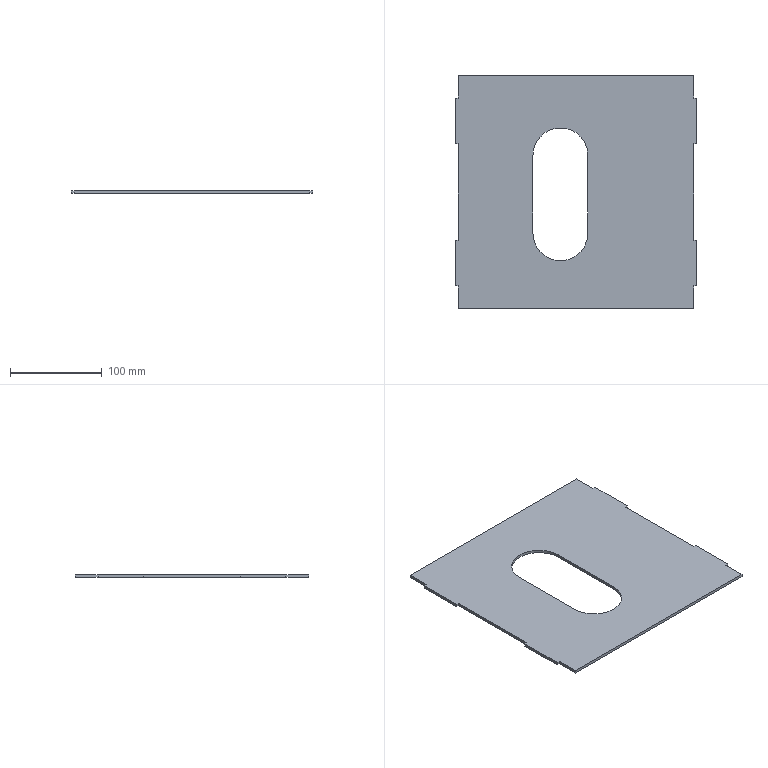Part | SolidWorks | features FlatPattern 1, SMBaseFlange 1, SheetMetal 1 | 1 solid | 26 faces | box 263.3 x 255 x 3.2 mm | volume 186509 mm3 | plane 24 | cylinder 2 | commonest cylinder face diameters 60 x2
STEP:
#1=CARTESIAN_POINT('',(-388.35,-199.918,0.));
#2=VERTEX_POINT('',#1);
#3=CARTESIAN_POINT('',(-388.35,-224.918,0.));
#4=VERTEX_POINT('',#3);
#5=CARTESIAN_POINT('',(-388.35,-224.918,0.));
#6=DIRECTION('',(0.,-1.,0.));
#7=VECTOR('',#6,1000.);
#8=LINE('',#5,#7);
#9=EDGE_CURVE('',#2,#4,#8,.T.);
#10=ORIENTED_EDGE('',*,*,#9,.F.);
#11=CARTESIAN_POINT('',(-388.35,-199.918,-3.2));
#12=VERTEX_POINT('',#11);
#13=CARTESIAN_POINT('',(-388.35,-199.918,-3.2));
#14=DIRECTION('',(0.,0.,1.));
#15=VECTOR('',#14,1000.);
#16=LINE('',#13,#15);
#17=EDGE_CURVE('',#12,#2,#16,.T.);
#18=ORIENTED_EDGE('',*,*,#17,.F.);
#19=CARTESIAN_POINT('',(-388.35,-224.918,-3.2));
#20=VERTEX_POINT('',#19);
#21=CARTESIAN_POINT('',(-388.35,-224.918,-3.2));
#22=DIRECTION('',(0.,-1.,0.));
#23=VECTOR('',#22,1000.);
#24=LINE('',#21,#23);
#25=EDGE_CURVE('',#12,#20,#24,.T.);
#26=ORIENTED_EDGE('',*,*,#25,.T.);
#27=CARTESIAN_POINT('',(-388.35,-224.918,-3.2));
#28=DIRECTION('',(0.,0.,1.));
#29=VECTOR('',#28,1000.);
#30=LINE('',#27,#29);
#31=EDGE_CURVE('',#20,#4,#30,.T.);
#32=ORIENTED_EDGE('',*,*,#31,.T.);
#33=EDGE_LOOP('',(#10,#18,#26,#32));
#34=FACE_OUTER_BOUND('',#33,.T.);
#35=CARTESIAN_POINT('',(-388.35,-224.918,-3.2));
#36=DIRECTION('',(-1.,0.,0.));
#37=DIRECTION('',(0.,0.,1.));
#38=AXIS2_PLACEMENT_3D('',#35,#36,#37);
#39=PLANE('',#38);
#40=ADVANCED_FACE('',(#34),#39,.T.);
#41=CARTESIAN_POINT('',(-391.35,-199.918,0.));
#42=VERTEX_POINT('',#41);
#43=CARTESIAN_POINT('',(-388.35,-199.918,0.));
#44=DIRECTION('',(1.,0.,0.));
#45=VECTOR('',#44,1000.);
#46=LINE('',#43,#45);
#47=EDGE_CURVE('',#42,#2,#46,.T.);
#48=ORIENTED_EDGE('',*,*,#47,.F.);
#49=CARTESIAN_POINT('',(-391.35,-199.918,-3.2));
#50=VERTEX_POINT('',#49);
#51=CARTESIAN_POINT('',(-391.35,-199.918,-3.2));
#52=DIRECTION('',(0.,0.,1.));
#53=VECTOR('',#52,1000.);
#54=LINE('',#51,#53);
#55=EDGE_CURVE('',#50,#42,#54,.T.);
#56=ORIENTED_EDGE('',*,*,#55,.F.);
#57=CARTESIAN_POINT('',(-388.35,-199.918,-3.2));
#58=DIRECTION('',(1.,0.,0.));
#59=VECTOR('',#58,1000.);
#60=LINE('',#57,#59);
#61=EDGE_CURVE('',#50,#12,#60,.T.);
#62=ORIENTED_EDGE('',*,*,#61,.T.);
#63=ORIENTED_EDGE('',*,*,#17,.T.);
#64=EDGE_LOOP('',(#48,#56,#62,#63));
#65=FACE_OUTER_BOUND('',#64,.T.);
#66=CARTESIAN_POINT('',(-388.35,-199.918,-3.2));
#67=DIRECTION('',(0.,-1.,0.));
#68=DIRECTION('',(0.,0.,-1.));
#69=AXIS2_PLACEMENT_3D('',#66,#67,#68);
#70=PLANE('',#69);
#71=ADVANCED_FACE('',(#65),#70,.T.);
#72=CARTESIAN_POINT('',(-391.35,-149.918,0.));
#73=VERTEX_POINT('',#72);
#74=CARTESIAN_POINT('',(-391.35,-199.918,0.));
#75=DIRECTION('',(0.,-1.,0.));
#76=VECTOR('',#75,1000.);
#77=LINE('',#74,#76);
#78=EDGE_CURVE('',#73,#42,#77,.T.);
#79=ORIENTED_EDGE('',*,*,#78,.F.);
#80=CARTESIAN_POINT('',(-391.35,-149.918,-3.2));
#81=VERTEX_POINT('',#80);
#82=CARTESIAN_POINT('',(-391.35,-149.918,-3.2));
#83=DIRECTION('',(0.,0.,1.));
#84=VECTOR('',#83,1000.);
#85=LINE('',#82,#84);
#86=EDGE_CURVE('',#81,#73,#85,.T.);
#87=ORIENTED_EDGE('',*,*,#86,.F.);
#88=CARTESIAN_POINT('',(-391.35,-199.918,-3.2));
#89=DIRECTION('',(0.,-1.,0.));
#90=VECTOR('',#89,1000.);
#91=LINE('',#88,#90);
#92=EDGE_CURVE('',#81,#50,#91,.T.);
#93=ORIENTED_EDGE('',*,*,#92,.T.);
#94=ORIENTED_EDGE('',*,*,#55,.T.);
#95=EDGE_LOOP('',(#79,#87,#93,#94));
#96=FACE_OUTER_BOUND('',#95,.T.);
#97=CARTESIAN_POINT('',(-391.35,-199.918,-3.2));
#98=DIRECTION('',(-1.,0.,0.));
#99=DIRECTION('',(0.,0.,1.));
#100=AXIS2_PLACEMENT_3D('',#97,#98,#99);
#101=PLANE('',#100);
#102=ADVANCED_FACE('',(#96),#101,.T.);
#103=CARTESIAN_POINT('',(-388.35,-149.918,0.));
#104=VERTEX_POINT('',#103);
#105=CARTESIAN_POINT('',(-391.35,-149.918,0.));
#106=DIRECTION('',(-1.,0.,0.));
#107=VECTOR('',#106,1000.);
#108=LINE('',#105,#107);
#109=EDGE_CURVE('',#104,#73,#108,.T.);
#110=ORIENTED_EDGE('',*,*,#109,.F.);
#111=CARTESIAN_POINT('',(-388.35,-149.918,-3.2));
#112=VERTEX_POINT('',#111);
#113=CARTESIAN_POINT('',(-388.35,-149.918,-3.2));
#114=DIRECTION('',(0.,0.,1.));
#115=VECTOR('',#114,1000.);
#116=LINE('',#113,#115);
#117=EDGE_CURVE('',#112,#104,#116,.T.);
#118=ORIENTED_EDGE('',*,*,#117,.F.);
#119=CARTESIAN_POINT('',(-391.35,-149.918,-3.2));
#120=DIRECTION('',(-1.,0.,0.));
#121=VECTOR('',#120,1000.);
#122=LINE('',#119,#121);
#123=EDGE_CURVE('',#112,#81,#122,.T.);
#124=ORIENTED_EDGE('',*,*,#123,.T.);
#125=ORIENTED_EDGE('',*,*,#86,.T.);
#126=EDGE_LOOP('',(#110,#118,#124,#125));
#127=FACE_OUTER_BOUND('',#126,.T.);
#128=CARTESIAN_POINT('',(-391.35,-149.918,-3.2));
#129=DIRECTION('',(0.,1.,0.));
#130=DIRECTION('',(0.,0.,1.));
#131=AXIS2_PLACEMENT_3D('',#128,#129,#130);
#132=PLANE('',#131);
#133=ADVANCED_FACE('',(#127),#132,.T.);
#134=CARTESIAN_POINT('',(-388.35,-44.918,0.));
#135=VERTEX_POINT('',#134);
#136=CARTESIAN_POINT('',(-388.35,-149.918,0.));
#137=DIRECTION('',(0.,-1.,0.));
#138=VECTOR('',#137,1000.);
#139=LINE('',#136,#138);
#140=EDGE_CURVE('',#135,#104,#139,.T.);
#141=ORIENTED_EDGE('',*,*,#140,.F.);
#142=CARTESIAN_POINT('',(-388.35,-44.918,-3.2));
#143=VERTEX_POINT('',#142);
#144=CARTESIAN_POINT('',(-388.35,-44.918,-3.2));
#145=DIRECTION('',(0.,0.,1.));
#146=VECTOR('',#145,1000.);
#147=LINE('',#144,#146);
#148=EDGE_CURVE('',#143,#135,#147,.T.);
#149=ORIENTED_EDGE('',*,*,#148,.F.);
#150=CARTESIAN_POINT('',(-388.35,-149.918,-3.2));
#151=DIRECTION('',(0.,-1.,0.));
#152=VECTOR('',#151,1000.);
#153=LINE('',#150,#152);
#154=EDGE_CURVE('',#143,#112,#153,.T.);
#155=ORIENTED_EDGE('',*,*,#154,.T.);
#156=ORIENTED_EDGE('',*,*,#117,.T.);
#157=EDGE_LOOP('',(#141,#149,#155,#156));
#158=FACE_OUTER_BOUND('',#157,.T.);
#159=CARTESIAN_POINT('',(-388.35,-149.918,-3.2));
#160=DIRECTION('',(-1.,0.,0.));
#161=DIRECTION('',(0.,0.,1.));
#162=AXIS2_PLACEMENT_3D('',#159,#160,#161);
#163=PLANE('',#162);
#164=ADVANCED_FACE('',(#158),#163,.T.);
#165=CARTESIAN_POINT('',(-391.35,-44.918,0.));
#166=VERTEX_POINT('',#165);
#167=CARTESIAN_POINT('',(-391.35,-44.918,0.));
#168=DIRECTION('',(1.,0.,0.));
#169=VECTOR('',#168,1000.);
#170=LINE('',#167,#169);
#171=EDGE_CURVE('',#166,#135,#170,.T.);
#172=ORIENTED_EDGE('',*,*,#171,.F.);
#173=CARTESIAN_POINT('',(-391.35,-44.918,-3.2));
#174=VERTEX_POINT('',#173);
#175=CARTESIAN_POINT('',(-391.35,-44.918,-3.2));
#176=DIRECTION('',(0.,0.,1.));
#177=VECTOR('',#176,1000.);
#178=LINE('',#175,#177);
#179=EDGE_CURVE('',#174,#166,#178,.T.);
#180=ORIENTED_EDGE('',*,*,#179,.F.);
#181=CARTESIAN_POINT('',(-391.35,-44.918,-3.2));
#182=DIRECTION('',(1.,0.,0.));
#183=VECTOR('',#182,1000.);
#184=LINE('',#181,#183);
#185=EDGE_CURVE('',#174,#143,#184,.T.);
#186=ORIENTED_EDGE('',*,*,#185,.T.);
#187=ORIENTED_EDGE('',*,*,#148,.T.);
#188=EDGE_LOOP('',(#172,#180,#186,#187));
#189=FACE_OUTER_BOUND('',#188,.T.);
#190=CARTESIAN_POINT('',(-391.35,-44.918,-3.2));
#191=DIRECTION('',(0.,-1.,0.));
#192=DIRECTION('',(0.,0.,-1.));
#193=AXIS2_PLACEMENT_3D('',#190,#191,#192);
#194=PLANE('',#193);
#195=ADVANCED_FACE('',(#189),#194,.T.);
#196=CARTESIAN_POINT('',(-391.35,5.082,0.));
#197=VERTEX_POINT('',#196);
#198=CARTESIAN_POINT('',(-391.35,5.082,0.));
#199=DIRECTION('',(0.,-1.,0.));
#200=VECTOR('',#199,1000.);
#201=LINE('',#198,#200);
#202=EDGE_CURVE('',#197,#166,#201,.T.);
#203=ORIENTED_EDGE('',*,*,#202,.F.);
#204=CARTESIAN_POINT('',(-391.35,5.082,-3.2));
#205=VERTEX_POINT('',#204);
#206=CARTESIAN_POINT('',(-391.35,5.082,-3.2));
#207=DIRECTION('',(0.,0.,1.));
#208=VECTOR('',#207,1000.);
#209=LINE('',#206,#208);
#210=EDGE_CURVE('',#205,#197,#209,.T.);
#211=ORIENTED_EDGE('',*,*,#210,.F.);
#212=CARTESIAN_POINT('',(-391.35,5.082,-3.2));
#213=DIRECTION('',(0.,-1.,0.));
#214=VECTOR('',#213,1000.);
#215=LINE('',#212,#214);
#216=EDGE_CURVE('',#205,#174,#215,.T.);
#217=ORIENTED_EDGE('',*,*,#216,.T.);
#218=ORIENTED_EDGE('',*,*,#179,.T.);
#219=EDGE_LOOP('',(#203,#211,#217,#218));
#220=FACE_OUTER_BOUND('',#219,.T.);
#221=CARTESIAN_POINT('',(-391.35,5.082,-3.2));
#222=DIRECTION('',(-1.,0.,0.));
#223=DIRECTION('',(0.,0.,1.));
#224=AXIS2_PLACEMENT_3D('',#221,#222,#223);
#225=PLANE('',#224);
#226=ADVANCED_FACE('',(#220),#225,.T.);
#227=CARTESIAN_POINT('',(-388.35,5.082,0.));
#228=VERTEX_POINT('',#227);
#229=CARTESIAN_POINT('',(-388.35,5.082,0.));
#230=DIRECTION('',(-1.,0.,0.));
#231=VECTOR('',#230,1000.);
#232=LINE('',#229,#231);
#233=EDGE_CURVE('',#228,#197,#232,.T.);
#234=ORIENTED_EDGE('',*,*,#233,.F.);
#235=CARTESIAN_POINT('',(-388.35,5.082,-3.2));
#236=VERTEX_POINT('',#235);
#237=CARTESIAN_POINT('',(-388.35,5.082,-3.2));
#238=DIRECTION('',(0.,0.,1.));
#239=VECTOR('',#238,1000.);
#240=LINE('',#237,#239);
#241=EDGE_CURVE('',#236,#228,#240,.T.);
#242=ORIENTED_EDGE('',*,*,#241,.F.);
#243=CARTESIAN_POINT('',(-388.35,5.082,-3.2));
#244=DIRECTION('',(-1.,0.,0.));
#245=VECTOR('',#244,1000.);
#246=LINE('',#243,#245);
#247=EDGE_CURVE('',#236,#205,#246,.T.);
#248=ORIENTED_EDGE('',*,*,#247,.T.);
#249=ORIENTED_EDGE('',*,*,#210,.T.);
#250=EDGE_LOOP('',(#234,#242,#248,#249));
#251=FACE_OUTER_BOUND('',#250,.T.);
#252=CARTESIAN_POINT('',(-388.35,5.082,-3.2));
#253=DIRECTION('',(0.,1.,0.));
#254=DIRECTION('',(0.,0.,1.));
#255=AXIS2_PLACEMENT_3D('',#252,#253,#254);
#256=PLANE('',#255);
#257=ADVANCED_FACE('',(#251),#256,.T.);
#258=CARTESIAN_POINT('',(-388.35,30.082,0.));
#259=VERTEX_POINT('',#258);
#260=CARTESIAN_POINT('',(-388.35,5.082,0.));
#261=DIRECTION('',(0.,-1.,0.));
#262=VECTOR('',#261,1000.);
#263=LINE('',#260,#262);
#264=EDGE_CURVE('',#259,#228,#263,.T.);
#265=ORIENTED_EDGE('',*,*,#264,.F.);
#266=CARTESIAN_POINT('',(-388.35,30.082,-3.2));
#267=VERTEX_POINT('',#266);
#268=CARTESIAN_POINT('',(-388.35,30.082,-3.2));
#269=DIRECTION('',(0.,0.,1.));
#270=VECTOR('',#269,1000.);
#271=LINE('',#268,#270);
#272=EDGE_CURVE('',#267,#259,#271,.T.);
#273=ORIENTED_EDGE('',*,*,#272,.F.);
#274=CARTESIAN_POINT('',(-388.35,5.082,-3.2));
#275=DIRECTION('',(0.,-1.,0.));
#276=VECTOR('',#275,1000.);
#277=LINE('',#274,#276);
#278=EDGE_CURVE('',#267,#236,#277,.T.);
#279=ORIENTED_EDGE('',*,*,#278,.T.);
#280=ORIENTED_EDGE('',*,*,#241,.T.);
#281=EDGE_LOOP('',(#265,#273,#279,#280));
#282=FACE_OUTER_BOUND('',#281,.T.);
#283=CARTESIAN_POINT('',(-388.35,5.082,-3.2));
#284=DIRECTION('',(-1.,0.,0.));
#285=DIRECTION('',(0.,0.,1.));
#286=AXIS2_PLACEMENT_3D('',#283,#284,#285);
#287=PLANE('',#286);
#288=ADVANCED_FACE('',(#282),#287,.T.);
#289=CARTESIAN_POINT('',(-131.05,30.082,0.));
#290=VERTEX_POINT('',#289);
#291=CARTESIAN_POINT('',(-388.35,30.082,0.));
#292=DIRECTION('',(-1.,0.,0.));
#293=VECTOR('',#292,1000.);
#294=LINE('',#291,#293);
#295=EDGE_CURVE('',#290,#259,#294,.T.);
#296=ORIENTED_EDGE('',*,*,#295,.F.);
#297=CARTESIAN_POINT('',(-131.05,30.082,-3.2));
#298=VERTEX_POINT('',#297);
#299=CARTESIAN_POINT('',(-131.05,30.082,-3.2));
#300=DIRECTION('',(0.,0.,1.));
#301=VECTOR('',#300,1000.);
#302=LINE('',#299,#301);
#303=EDGE_CURVE('',#298,#290,#302,.T.);
#304=ORIENTED_EDGE('',*,*,#303,.F.);
#305=CARTESIAN_POINT('',(-388.35,30.082,-3.2));
#306=DIRECTION('',(-1.,0.,0.));
#307=VECTOR('',#306,1000.);
#308=LINE('',#305,#307);
#309=EDGE_CURVE('',#298,#267,#308,.T.);
#310=ORIENTED_EDGE('',*,*,#309,.T.);
#311=ORIENTED_EDGE('',*,*,#272,.T.);
#312=EDGE_LOOP('',(#296,#304,#310,#311));
#313=FACE_OUTER_BOUND('',#312,.T.);
#314=CARTESIAN_POINT('',(-388.35,30.082,-3.2));
#315=DIRECTION('',(0.,1.,0.));
#316=DIRECTION('',(0.,0.,1.));
#317=AXIS2_PLACEMENT_3D('',#314,#315,#316);
#318=PLANE('',#317);
#319=ADVANCED_FACE('',(#313),#318,.T.);
#320=CARTESIAN_POINT('',(-131.05,5.082,0.));
#321=VERTEX_POINT('',#320);
#322=CARTESIAN_POINT('',(-131.05,5.082,0.));
#323=DIRECTION('',(0.,1.,0.));
#324=VECTOR('',#323,1000.);
#325=LINE('',#322,#324);
#326=EDGE_CURVE('',#321,#290,#325,.T.);
#327=ORIENTED_EDGE('',*,*,#326,.F.);
#328=CARTESIAN_POINT('',(-131.05,5.082,-3.2));
#329=VERTEX_POINT('',#328);
#330=CARTESIAN_POINT('',(-131.05,5.082,-3.2));
#331=DIRECTION('',(0.,0.,1.));
#332=VECTOR('',#331,1000.);
#333=LINE('',#330,#332);
#334=EDGE_CURVE('',#329,#321,#333,.T.);
#335=ORIENTED_EDGE('',*,*,#334,.F.);
#336=CARTESIAN_POINT('',(-131.05,5.082,-3.2));
#337=DIRECTION('',(0.,1.,0.));
#338=VECTOR('',#337,1000.);
#339=LINE('',#336,#338);
#340=EDGE_CURVE('',#329,#298,#339,.T.);
#341=ORIENTED_EDGE('',*,*,#340,.T.);
#342=ORIENTED_EDGE('',*,*,#303,.T.);
#343=EDGE_LOOP('',(#327,#335,#341,#342));
#344=FACE_OUTER_BOUND('',#343,.T.);
#345=CARTESIAN_POINT('',(-131.05,5.082,-3.2));
#346=DIRECTION('',(1.,0.,0.));
#347=DIRECTION('',(0.,0.,-1.));
#348=AXIS2_PLACEMENT_3D('',#345,#346,#347);
#349=PLANE('',#348);
#350=ADVANCED_FACE('',(#344),#349,.T.);
#351=CARTESIAN_POINT('',(-128.05,5.082,0.));
#352=VERTEX_POINT('',#351);
#353=CARTESIAN_POINT('',(-131.05,5.082,0.));
#354=DIRECTION('',(-1.,0.,0.));
#355=VECTOR('',#354,1000.);
#356=LINE('',#353,#355);
#357=EDGE_CURVE('',#352,#321,#356,.T.);
#358=ORIENTED_EDGE('',*,*,#357,.F.);
#359=CARTESIAN_POINT('',(-128.05,5.082,-3.2));
#360=VERTEX_POINT('',#359);
#361=CARTESIAN_POINT('',(-128.05,5.082,-3.2));
#362=DIRECTION('',(0.,0.,1.));
#363=VECTOR('',#362,1000.);
#364=LINE('',#361,#363);
#365=EDGE_CURVE('',#360,#352,#364,.T.);
#366=ORIENTED_EDGE('',*,*,#365,.F.);
#367=CARTESIAN_POINT('',(-131.05,5.082,-3.2));
#368=DIRECTION('',(-1.,0.,0.));
#369=VECTOR('',#368,1000.);
#370=LINE('',#367,#369);
#371=EDGE_CURVE('',#360,#329,#370,.T.);
#372=ORIENTED_EDGE('',*,*,#371,.T.);
#373=ORIENTED_EDGE('',*,*,#334,.T.);
#374=EDGE_LOOP('',(#358,#366,#372,#373));
#375=FACE_OUTER_BOUND('',#374,.T.);
#376=CARTESIAN_POINT('',(-131.05,5.082,-3.2));
#377=DIRECTION('',(0.,1.,0.));
#378=DIRECTION('',(0.,0.,1.));
#379=AXIS2_PLACEMENT_3D('',#376,#377,#378);
#380=PLANE('',#379);
#381=ADVANCED_FACE('',(#375),#380,.T.);
#382=CARTESIAN_POINT('',(-128.05,-44.918,0.));
#383=VERTEX_POINT('',#382);
#384=CARTESIAN_POINT('',(-128.05,5.082,0.));
#385=DIRECTION('',(0.,1.,0.));
#386=VECTOR('',#385,1000.);
#387=LINE('',#384,#386);
#388=EDGE_CURVE('',#383,#352,#387,.T.);
#389=ORIENTED_EDGE('',*,*,#388,.F.);
#390=CARTESIAN_POINT('',(-128.05,-44.918,-3.2));
#391=VERTEX_POINT('',#390);
#392=CARTESIAN_POINT('',(-128.05,-44.918,-3.2));
#393=DIRECTION('',(0.,0.,1.));
#394=VECTOR('',#393,1000.);
#395=LINE('',#392,#394);
#396=EDGE_CURVE('',#391,#383,#395,.T.);
#397=ORIENTED_EDGE('',*,*,#396,.F.);
#398=CARTESIAN_POINT('',(-128.05,5.082,-3.2));
#399=DIRECTION('',(0.,1.,0.));
#400=VECTOR('',#399,1000.);
#401=LINE('',#398,#400);
#402=EDGE_CURVE('',#391,#360,#401,.T.);
#403=ORIENTED_EDGE('',*,*,#402,.T.);
#404=ORIENTED_EDGE('',*,*,#365,.T.);
#405=EDGE_LOOP('',(#389,#397,#403,#404));
#406=FACE_OUTER_BOUND('',#405,.T.);
#407=CARTESIAN_POINT('',(-128.05,5.082,-3.2));
#408=DIRECTION('',(1.,0.,0.));
#409=DIRECTION('',(0.,0.,-1.));
#410=AXIS2_PLACEMENT_3D('',#407,#408,#409);
#411=PLANE('',#410);
#412=ADVANCED_FACE('',(#406),#411,.T.);
#413=CARTESIAN_POINT('',(-131.05,-44.918,0.));
#414=VERTEX_POINT('',#413);
#415=CARTESIAN_POINT('',(-128.05,-44.918,0.));
#416=DIRECTION('',(1.,0.,0.));
#417=VECTOR('',#416,1000.);
#418=LINE('',#415,#417);
#419=EDGE_CURVE('',#414,#383,#418,.T.);
#420=ORIENTED_EDGE('',*,*,#419,.F.);
#421=CARTESIAN_POINT('',(-131.05,-44.918,-3.2));
#422=VERTEX_POINT('',#421);
#423=CARTESIAN_POINT('',(-131.05,-44.918,-3.2));
#424=DIRECTION('',(0.,0.,1.));
#425=VECTOR('',#424,1000.);
#426=LINE('',#423,#425);
#427=EDGE_CURVE('',#422,#414,#426,.T.);
#428=ORIENTED_EDGE('',*,*,#427,.F.);
#429=CARTESIAN_POINT('',(-128.05,-44.918,-3.2));
#430=DIRECTION('',(1.,0.,0.));
#431=VECTOR('',#430,1000.);
#432=LINE('',#429,#431);
#433=EDGE_CURVE('',#422,#391,#432,.T.);
#434=ORIENTED_EDGE('',*,*,#433,.T.);
#435=ORIENTED_EDGE('',*,*,#396,.T.);
#436=EDGE_LOOP('',(#420,#428,#434,#435));
#437=FACE_OUTER_BOUND('',#436,.T.);
#438=CARTESIAN_POINT('',(-128.05,-44.918,-3.2));
#439=DIRECTION('',(0.,-1.,0.));
#440=DIRECTION('',(0.,0.,-1.));
#441=AXIS2_PLACEMENT_3D('',#438,#439,#440);
#442=PLANE('',#441);
#443=ADVANCED_FACE('',(#437),#442,.T.);
#444=CARTESIAN_POINT('',(-131.05,-149.918,0.));
#445=VERTEX_POINT('',#444);
#446=CARTESIAN_POINT('',(-131.05,-149.918,0.));
#447=DIRECTION('',(0.,1.,0.));
#448=VECTOR('',#447,1000.);
#449=LINE('',#446,#448);
#450=EDGE_CURVE('',#445,#414,#449,.T.);
#451=ORIENTED_EDGE('',*,*,#450,.F.);
#452=CARTESIAN_POINT('',(-131.05,-149.918,-3.2));
#453=VERTEX_POINT('',#452);
#454=CARTESIAN_POINT('',(-131.05,-149.918,-3.2));
#455=DIRECTION('',(0.,0.,1.));
#456=VECTOR('',#455,1000.);
#457=LINE('',#454,#456);
#458=EDGE_CURVE('',#453,#445,#457,.T.);
#459=ORIENTED_EDGE('',*,*,#458,.F.);
#460=CARTESIAN_POINT('',(-131.05,-149.918,-3.2));
#461=DIRECTION('',(0.,1.,0.));
#462=VECTOR('',#461,1000.);
#463=LINE('',#460,#462);
#464=EDGE_CURVE('',#453,#422,#463,.T.);
#465=ORIENTED_EDGE('',*,*,#464,.T.);
#466=ORIENTED_EDGE('',*,*,#427,.T.);
#467=EDGE_LOOP('',(#451,#459,#465,#466));
#468=FACE_OUTER_BOUND('',#467,.T.);
#469=CARTESIAN_POINT('',(-131.05,-149.918,-3.2));
#470=DIRECTION('',(1.,0.,0.));
#471=DIRECTION('',(0.,0.,-1.));
#472=AXIS2_PLACEMENT_3D('',#469,#470,#471);
#473=PLANE('',#472);
#474=ADVANCED_FACE('',(#468),#473,.T.);
#475=CARTESIAN_POINT('',(-128.05,-149.918,0.));
#476=VERTEX_POINT('',#475);
#477=CARTESIAN_POINT('',(-128.05,-149.918,0.));
#478=DIRECTION('',(-1.,0.,0.));
#479=VECTOR('',#478,1000.);
#480=LINE('',#477,#479);
#481=EDGE_CURVE('',#476,#445,#480,.T.);
#482=ORIENTED_EDGE('',*,*,#481,.F.);
#483=CARTESIAN_POINT('',(-128.05,-149.918,-3.2));
#484=VERTEX_POINT('',#483);
#485=CARTESIAN_POINT('',(-128.05,-149.918,-3.2));
#486=DIRECTION('',(0.,0.,1.));
#487=VECTOR('',#486,1000.);
#488=LINE('',#485,#487);
#489=EDGE_CURVE('',#484,#476,#488,.T.);
#490=ORIENTED_EDGE('',*,*,#489,.F.);
#491=CARTESIAN_POINT('',(-128.05,-149.918,-3.2));
#492=DIRECTION('',(-1.,0.,0.));
#493=VECTOR('',#492,1000.);
#494=LINE('',#491,#493);
#495=EDGE_CURVE('',#484,#453,#494,.T.);
#496=ORIENTED_EDGE('',*,*,#495,.T.);
#497=ORIENTED_EDGE('',*,*,#458,.T.);
#498=EDGE_LOOP('',(#482,#490,#496,#497));
#499=FACE_OUTER_BOUND('',#498,.T.);
#500=CARTESIAN_POINT('',(-128.05,-149.918,-3.2));
#501=DIRECTION('',(0.,1.,0.));
#502=DIRECTION('',(0.,0.,1.));
#503=AXIS2_PLACEMENT_3D('',#500,#501,#502);
#504=PLANE('',#503);
#505=ADVANCED_FACE('',(#499),#504,.T.);
#506=CARTESIAN_POINT('',(-128.05,-199.918,0.));
#507=VERTEX_POINT('',#506);
#508=CARTESIAN_POINT('',(-128.05,-199.918,0.));
#509=DIRECTION('',(0.,1.,0.));
#510=VECTOR('',#509,1000.);
#511=LINE('',#508,#510);
#512=EDGE_CURVE('',#507,#476,#511,.T.);
#513=ORIENTED_EDGE('',*,*,#512,.F.);
#514=CARTESIAN_POINT('',(-128.05,-199.918,-3.2));
#515=VERTEX_POINT('',#514);
#516=CARTESIAN_POINT('',(-128.05,-199.918,-3.2));
#517=DIRECTION('',(0.,0.,1.));
#518=VECTOR('',#517,1000.);
#519=LINE('',#516,#518);
#520=EDGE_CURVE('',#515,#507,#519,.T.);
#521=ORIENTED_EDGE('',*,*,#520,.F.);
#522=CARTESIAN_POINT('',(-128.05,-199.918,-3.2));
#523=DIRECTION('',(0.,1.,0.));
#524=VECTOR('',#523,1000.);
#525=LINE('',#522,#524);
#526=EDGE_CURVE('',#515,#484,#525,.T.);
#527=ORIENTED_EDGE('',*,*,#526,.T.);
#528=ORIENTED_EDGE('',*,*,#489,.T.);
#529=EDGE_LOOP('',(#513,#521,#527,#528));
#530=FACE_OUTER_BOUND('',#529,.T.);
#531=CARTESIAN_POINT('',(-128.05,-199.918,-3.2));
#532=DIRECTION('',(1.,0.,0.));
#533=DIRECTION('',(0.,0.,-1.));
#534=AXIS2_PLACEMENT_3D('',#531,#532,#533);
#535=PLANE('',#534);
#536=ADVANCED_FACE('',(#530),#535,.T.);
#537=CARTESIAN_POINT('',(-131.05,-199.918,0.));
#538=VERTEX_POINT('',#537);
#539=CARTESIAN_POINT('',(-131.05,-199.918,0.));
#540=DIRECTION('',(1.,0.,0.));
#541=VECTOR('',#540,1000.);
#542=LINE('',#539,#541);
#543=EDGE_CURVE('',#538,#507,#542,.T.);
#544=ORIENTED_EDGE('',*,*,#543,.F.);
#545=CARTESIAN_POINT('',(-131.05,-199.918,-3.2));
#546=VERTEX_POINT('',#545);
#547=CARTESIAN_POINT('',(-131.05,-199.918,-3.2));
#548=DIRECTION('',(0.,0.,1.));
#549=VECTOR('',#548,1000.);
#550=LINE('',#547,#549);
#551=EDGE_CURVE('',#546,#538,#550,.T.);
#552=ORIENTED_EDGE('',*,*,#551,.F.);
#553=CARTESIAN_POINT('',(-131.05,-199.918,-3.2));
#554=DIRECTION('',(1.,0.,0.));
#555=VECTOR('',#554,1000.);
#556=LINE('',#553,#555);
#557=EDGE_CURVE('',#546,#515,#556,.T.);
#558=ORIENTED_EDGE('',*,*,#557,.T.);
#559=ORIENTED_EDGE('',*,*,#520,.T.);
#560=EDGE_LOOP('',(#544,#552,#558,#559));
#561=FACE_OUTER_BOUND('',#560,.T.);
#562=CARTESIAN_POINT('',(-131.05,-199.918,-3.2));
#563=DIRECTION('',(0.,-1.,0.));
#564=DIRECTION('',(0.,0.,-1.));
#565=AXIS2_PLACEMENT_3D('',#562,#563,#564);
#566=PLANE('',#565);
#567=ADVANCED_FACE('',(#561),#566,.T.);
#568=CARTESIAN_POINT('',(-131.05,-224.918,0.));
#569=VERTEX_POINT('',#568);
#570=CARTESIAN_POINT('',(-131.05,-224.918,0.));
#571=DIRECTION('',(0.,1.,0.));
#572=VECTOR('',#571,1000.);
#573=LINE('',#570,#572);
#574=EDGE_CURVE('',#569,#538,#573,.T.);
#575=ORIENTED_EDGE('',*,*,#574,.F.);
#576=CARTESIAN_POINT('',(-131.05,-224.918,-3.2));
#577=VERTEX_POINT('',#576);
#578=CARTESIAN_POINT('',(-131.05,-224.918,-3.2));
#579=DIRECTION('',(0.,0.,1.));
#580=VECTOR('',#579,1000.);
#581=LINE('',#578,#580);
#582=EDGE_CURVE('',#577,#569,#581,.T.);
#583=ORIENTED_EDGE('',*,*,#582,.F.);
#584=CARTESIAN_POINT('',(-131.05,-224.918,-3.2));
#585=DIRECTION('',(0.,1.,0.));
#586=VECTOR('',#585,1000.);
#587=LINE('',#584,#586);
#588=EDGE_CURVE('',#577,#546,#587,.T.);
#589=ORIENTED_EDGE('',*,*,#588,.T.);
#590=ORIENTED_EDGE('',*,*,#551,.T.);
#591=EDGE_LOOP('',(#575,#583,#589,#590));
#592=FACE_OUTER_BOUND('',#591,.T.);
#593=CARTESIAN_POINT('',(-131.05,-224.918,-3.2));
#594=DIRECTION('',(1.,0.,0.));
#595=DIRECTION('',(0.,0.,-1.));
#596=AXIS2_PLACEMENT_3D('',#593,#594,#595);
#597=PLANE('',#596);
#598=ADVANCED_FACE('',(#592),#597,.T.);
#599=CARTESIAN_POINT('',(-388.35,-224.918,0.));
#600=DIRECTION('',(1.,0.,0.));
#601=VECTOR('',#600,1000.);
#602=LINE('',#599,#601);
#603=EDGE_CURVE('',#4,#569,#602,.T.);
#604=ORIENTED_EDGE('',*,*,#603,.F.);
#605=ORIENTED_EDGE('',*,*,#31,.F.);
#606=CARTESIAN_POINT('',(-388.35,-224.918,-3.2));
#607=DIRECTION('',(1.,0.,0.));
#608=VECTOR('',#607,1000.);
#609=LINE('',#606,#608);
#610=EDGE_CURVE('',#20,#577,#609,.T.);
#611=ORIENTED_EDGE('',*,*,#610,.T.);
#612=ORIENTED_EDGE('',*,*,#582,.T.);
#613=EDGE_LOOP('',(#604,#605,#611,#612));
#614=FACE_OUTER_BOUND('',#613,.T.);
#615=CARTESIAN_POINT('',(-388.35,-224.918,-3.2));
#616=DIRECTION('',(0.,-1.,0.));
#617=DIRECTION('',(0.,0.,-1.));
#618=AXIS2_PLACEMENT_3D('',#615,#616,#617);
#619=PLANE('',#618);
#620=ADVANCED_FACE('',(#614),#619,.T.);
#621=CARTESIAN_POINT('',(-306.65,-57.418,-3.2));
#622=VERTEX_POINT('',#621);
#623=CARTESIAN_POINT('',(-306.65,-142.418,-3.2));
#624=VERTEX_POINT('',#623);
#625=CARTESIAN_POINT('',(-306.65,-142.418,-3.2));
#626=DIRECTION('',(0.,-1.,0.));
#627=VECTOR('',#626,1000.);
#628=LINE('',#625,#627);
#629=EDGE_CURVE('',#622,#624,#628,.T.);
#630=ORIENTED_EDGE('',*,*,#629,.T.);
#631=CARTESIAN_POINT('',(-246.65,-142.418,-3.2));
#632=VERTEX_POINT('',#631);
#633=CARTESIAN_POINT('',(-276.65,-142.418,-3.2));
#634=DIRECTION('',(0.,0.,1.));
#635=DIRECTION('',(1.,0.,0.));
#636=AXIS2_PLACEMENT_3D('',#633,#634,#635);
#637=CIRCLE('',#636,30.);
#638=EDGE_CURVE('',#624,#632,#637,.T.);
#639=ORIENTED_EDGE('',*,*,#638,.T.);
#640=CARTESIAN_POINT('',(-246.65,-57.418,-3.2));
#641=VERTEX_POINT('',#640);
#642=CARTESIAN_POINT('',(-246.65,-142.418,-3.2));
#643=DIRECTION('',(0.,1.,0.));
#644=VECTOR('',#643,1000.);
#645=LINE('',#642,#644);
#646=EDGE_CURVE('',#632,#641,#645,.T.);
#647=ORIENTED_EDGE('',*,*,#646,.T.);
#648=CARTESIAN_POINT('',(-276.65,-57.418,-3.2));
#649=DIRECTION('',(0.,0.,1.));
#650=DIRECTION('',(1.,0.,0.));
#651=AXIS2_PLACEMENT_3D('',#648,#649,#650);
#652=CIRCLE('',#651,30.);
#653=EDGE_CURVE('',#641,#622,#652,.T.);
#654=ORIENTED_EDGE('',*,*,#653,.T.);
#655=EDGE_LOOP('',(#630,#639,#647,#654));
#656=FACE_BOUND('',#655,.T.);
#657=ORIENTED_EDGE('',*,*,#25,.F.);
#658=ORIENTED_EDGE('',*,*,#61,.F.);
#659=ORIENTED_EDGE('',*,*,#92,.F.);
#660=ORIENTED_EDGE('',*,*,#123,.F.);
#661=ORIENTED_EDGE('',*,*,#154,.F.);
#662=ORIENTED_EDGE('',*,*,#185,.F.);
#663=ORIENTED_EDGE('',*,*,#216,.F.);
#664=ORIENTED_EDGE('',*,*,#247,.F.);
#665=ORIENTED_EDGE('',*,*,#278,.F.);
#666=ORIENTED_EDGE('',*,*,#309,.F.);
#667=ORIENTED_EDGE('',*,*,#340,.F.);
#668=ORIENTED_EDGE('',*,*,#371,.F.);
#669=ORIENTED_EDGE('',*,*,#402,.F.);
#670=ORIENTED_EDGE('',*,*,#433,.F.);
#671=ORIENTED_EDGE('',*,*,#464,.F.);
#672=ORIENTED_EDGE('',*,*,#495,.F.);
#673=ORIENTED_EDGE('',*,*,#526,.F.);
#674=ORIENTED_EDGE('',*,*,#557,.F.);
#675=ORIENTED_EDGE('',*,*,#588,.F.);
#676=ORIENTED_EDGE('',*,*,#610,.F.);
#677=EDGE_LOOP('',(#657,#658,#659,#660,#661,#662,#663,#664,#665,#666,#667,#668,#669,#670,#671,#672,#673,#674,#675,#676));
#678=FACE_OUTER_BOUND('',#677,.T.);
#679=CARTESIAN_POINT('',(0.,0.,-3.2));
#680=DIRECTION('',(0.,0.,1.));
#681=DIRECTION('',(1.,0.,0.));
#682=AXIS2_PLACEMENT_3D('',#679,#680,#681);
#683=PLANE('',#682);
#684=ADVANCED_FACE('',(#656,#678),#683,.F.);
#685=CARTESIAN_POINT('',(-306.65,-142.418,0.));
#686=VERTEX_POINT('',#685);
#687=CARTESIAN_POINT('',(-246.65,-142.418,0.));
#688=VERTEX_POINT('',#687);
#689=CARTESIAN_POINT('',(-276.65,-142.418,0.));
#690=DIRECTION('',(0.,0.,1.));
#691=DIRECTION('',(1.,0.,0.));
#692=AXIS2_PLACEMENT_3D('',#689,#690,#691);
#693=CIRCLE('',#692,30.);
#694=EDGE_CURVE('',#686,#688,#693,.T.);
#695=ORIENTED_EDGE('',*,*,#694,.F.);
#696=CARTESIAN_POINT('',(-306.65,-57.418,0.));
#697=VERTEX_POINT('',#696);
#698=CARTESIAN_POINT('',(-306.65,-142.418,0.));
#699=DIRECTION('',(0.,-1.,0.));
#700=VECTOR('',#699,1000.);
#701=LINE('',#698,#700);
#702=EDGE_CURVE('',#697,#686,#701,.T.);
#703=ORIENTED_EDGE('',*,*,#702,.F.);
#704=CARTESIAN_POINT('',(-246.65,-57.418,0.));
#705=VERTEX_POINT('',#704);
#706=CARTESIAN_POINT('',(-276.65,-57.418,0.));
#707=DIRECTION('',(0.,0.,1.));
#708=DIRECTION('',(1.,0.,0.));
#709=AXIS2_PLACEMENT_3D('',#706,#707,#708);
#710=CIRCLE('',#709,30.);
#711=EDGE_CURVE('',#705,#697,#710,.T.);
#712=ORIENTED_EDGE('',*,*,#711,.F.);
#713=CARTESIAN_POINT('',(-246.65,-142.418,0.));
#714=DIRECTION('',(0.,1.,0.));
#715=VECTOR('',#714,1000.);
#716=LINE('',#713,#715);
#717=EDGE_CURVE('',#688,#705,#716,.T.);
#718=ORIENTED_EDGE('',*,*,#717,.F.);
#719=EDGE_LOOP('',(#695,#703,#712,#718));
#720=FACE_BOUND('',#719,.T.);
#721=ORIENTED_EDGE('',*,*,#9,.T.);
#722=ORIENTED_EDGE('',*,*,#603,.T.);
#723=ORIENTED_EDGE('',*,*,#574,.T.);
#724=ORIENTED_EDGE('',*,*,#543,.T.);
#725=ORIENTED_EDGE('',*,*,#512,.T.);
#726=ORIENTED_EDGE('',*,*,#481,.T.);
#727=ORIENTED_EDGE('',*,*,#450,.T.);
#728=ORIENTED_EDGE('',*,*,#419,.T.);
#729=ORIENTED_EDGE('',*,*,#388,.T.);
#730=ORIENTED_EDGE('',*,*,#357,.T.);
#731=ORIENTED_EDGE('',*,*,#326,.T.);
#732=ORIENTED_EDGE('',*,*,#295,.T.);
#733=ORIENTED_EDGE('',*,*,#264,.T.);
#734=ORIENTED_EDGE('',*,*,#233,.T.);
#735=ORIENTED_EDGE('',*,*,#202,.T.);
#736=ORIENTED_EDGE('',*,*,#171,.T.);
#737=ORIENTED_EDGE('',*,*,#140,.T.);
#738=ORIENTED_EDGE('',*,*,#109,.T.);
#739=ORIENTED_EDGE('',*,*,#78,.T.);
#740=ORIENTED_EDGE('',*,*,#47,.T.);
#741=EDGE_LOOP('',(#721,#722,#723,#724,#725,#726,#727,#728,#729,#730,#731,#732,#733,#734,#735,#736,#737,#738,#739,#740));
#742=FACE_OUTER_BOUND('',#741,.T.);
#743=CARTESIAN_POINT('',(0.,0.,0.));
#744=DIRECTION('',(0.,0.,1.));
#745=DIRECTION('',(1.,0.,0.));
#746=AXIS2_PLACEMENT_3D('',#743,#744,#745);
#747=PLANE('',#746);
#748=ADVANCED_FACE('',(#720,#742),#747,.T.);
#749=ORIENTED_EDGE('',*,*,#694,.T.);
#750=CARTESIAN_POINT('',(-246.65,-142.418,-3.2));
#751=DIRECTION('',(0.,0.,1.));
#752=VECTOR('',#751,1000.);
#753=LINE('',#750,#752);
#754=EDGE_CURVE('',#632,#688,#753,.T.);
#755=ORIENTED_EDGE('',*,*,#754,.F.);
#756=ORIENTED_EDGE('',*,*,#638,.F.);
#757=CARTESIAN_POINT('',(-306.65,-142.418,-3.2));
#758=DIRECTION('',(0.,0.,1.));
#759=VECTOR('',#758,1000.);
#760=LINE('',#757,#759);
#761=EDGE_CURVE('',#624,#686,#760,.T.);
#762=ORIENTED_EDGE('',*,*,#761,.T.);
#763=EDGE_LOOP('',(#749,#755,#756,#762));
#764=FACE_OUTER_BOUND('',#763,.T.);
#765=CARTESIAN_POINT('',(-276.65,-142.418,-3.2));
#766=DIRECTION('',(0.,0.,1.));
#767=DIRECTION('',(1.,0.,0.));
#768=AXIS2_PLACEMENT_3D('',#765,#766,#767);
#769=CYLINDRICAL_SURFACE('',#768,30.);
#770=ADVANCED_FACE('',(#764),#769,.F.);
#771=ORIENTED_EDGE('',*,*,#702,.T.);
#772=ORIENTED_EDGE('',*,*,#761,.F.);
#773=ORIENTED_EDGE('',*,*,#629,.F.);
#774=CARTESIAN_POINT('',(-306.65,-57.418,-3.2));
#775=DIRECTION('',(0.,0.,1.));
#776=VECTOR('',#775,1000.);
#777=LINE('',#774,#776);
#778=EDGE_CURVE('',#622,#697,#777,.T.);
#779=ORIENTED_EDGE('',*,*,#778,.T.);
#780=EDGE_LOOP('',(#771,#772,#773,#779));
#781=FACE_OUTER_BOUND('',#780,.T.);
#782=CARTESIAN_POINT('',(-306.65,-142.418,-3.2));
#783=DIRECTION('',(-1.,0.,0.));
#784=DIRECTION('',(0.,0.,1.));
#785=AXIS2_PLACEMENT_3D('',#782,#783,#784);
#786=PLANE('',#785);
#787=ADVANCED_FACE('',(#781),#786,.F.);
#788=ORIENTED_EDGE('',*,*,#711,.T.);
#789=ORIENTED_EDGE('',*,*,#778,.F.);
#790=ORIENTED_EDGE('',*,*,#653,.F.);
#791=CARTESIAN_POINT('',(-246.65,-57.418,-3.2));
#792=DIRECTION('',(0.,0.,1.));
#793=VECTOR('',#792,1000.);
#794=LINE('',#791,#793);
#795=EDGE_CURVE('',#641,#705,#794,.T.);
#796=ORIENTED_EDGE('',*,*,#795,.T.);
#797=EDGE_LOOP('',(#788,#789,#790,#796));
#798=FACE_OUTER_BOUND('',#797,.T.);
#799=CARTESIAN_POINT('',(-276.65,-57.418,-3.2));
#800=DIRECTION('',(0.,0.,1.));
#801=DIRECTION('',(1.,0.,0.));
#802=AXIS2_PLACEMENT_3D('',#799,#800,#801);
#803=CYLINDRICAL_SURFACE('',#802,30.);
#804=ADVANCED_FACE('',(#798),#803,.F.);
#805=ORIENTED_EDGE('',*,*,#717,.T.);
#806=ORIENTED_EDGE('',*,*,#795,.F.);
#807=ORIENTED_EDGE('',*,*,#646,.F.);
#808=ORIENTED_EDGE('',*,*,#754,.T.);
#809=EDGE_LOOP('',(#805,#806,#807,#808));
#810=FACE_OUTER_BOUND('',#809,.T.);
#811=CARTESIAN_POINT('',(-246.65,-142.418,-3.2));
#812=DIRECTION('',(1.,0.,0.));
#813=DIRECTION('',(0.,1.,0.));
#814=AXIS2_PLACEMENT_3D('',#811,#812,#813);
#815=PLANE('',#814);
#816=ADVANCED_FACE('',(#810),#815,.F.);
#817=CLOSED_SHELL('',(#40,#71,#102,#133,#164,#195,#226,#257,#288,#319,#350,#381,#412,#443,#474,#505,#536,#567,#598,#620,#684,#748,#770,#787,#804,#816));
#818=MANIFOLD_SOLID_BREP('',#817);
#819=CARTESIAN_POINT('',(0.,0.,0.));
#820=DIRECTION('',(0.,0.,1.));
#821=DIRECTION('',(1.,0.,0.));
#822=AXIS2_PLACEMENT_3D('',#819,#820,#821);
#823=(LENGTH_UNIT()NAMED_UNIT(*)SI_UNIT(.MILLI.,.METRE.));
#824=UNCERTAINTY_MEASURE_WITH_UNIT(LENGTH_MEASURE(0.00001),#823,'','');
#825=(NAMED_UNIT(*)PLANE_ANGLE_UNIT()SI_UNIT($,.RADIAN.));
#826=(NAMED_UNIT(*)SI_UNIT($,.STERADIAN.)SOLID_ANGLE_UNIT());
#827=(GEOMETRIC_REPRESENTATION_CONTEXT(3)GLOBAL_UNCERTAINTY_ASSIGNED_CONTEXT((#824))GLOBAL_UNIT_ASSIGNED_CONTEXT((#823,#825,#826))REPRESENTATION_CONTEXT('',''));
#828=ADVANCED_BREP_SHAPE_REPRESENTATION('',(#818,#822),#827);